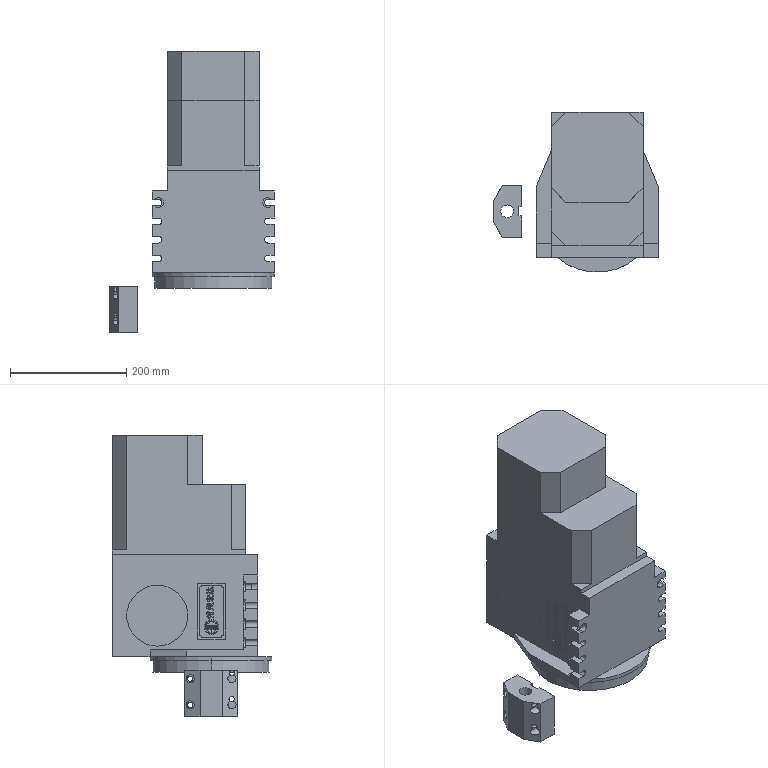Part | STEP file | HAK32080 Outline | 5 solids | 414 faces | box 283 x 275 x 483.5 mm | volume 14482459 mm3 | plane 266 | cylinder 93 | spline 49 | cone 6 | commonest cylinder face diameters 9 x12 14 x10 6 x8 11 x8 18 x8 21.138 x7